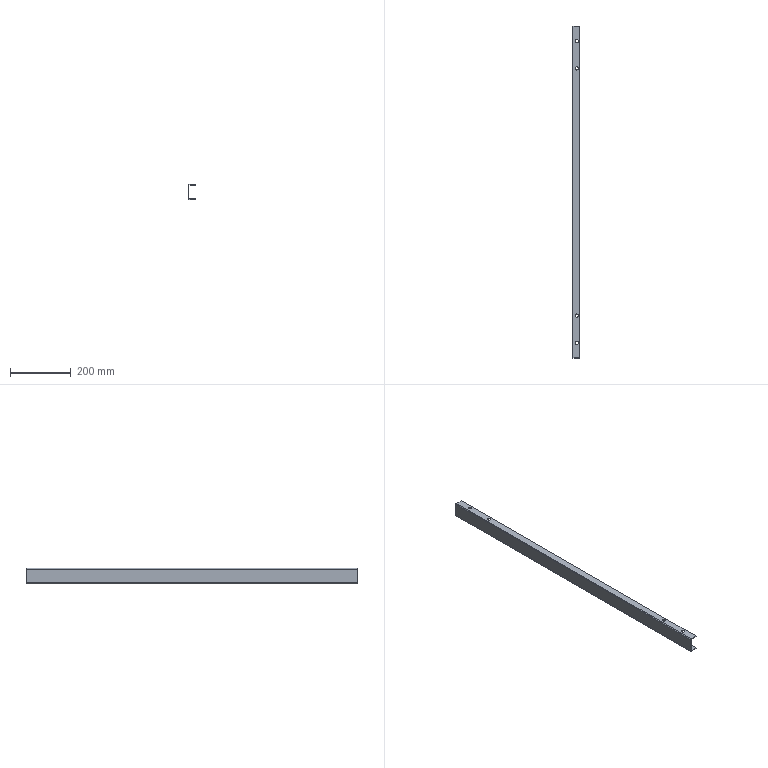Part | 1 solid | 38 faces | box 25 x 1096 x 50 mm | volume 206654 mm3 | cylinder 20 | plane 18 | commonest cylinder face diameters 11 x16 0.4 x2 4.4 x2
STEP:
#1=CARTESIAN_POINT('',(20.5,498.,-23.));
#2=VERTEX_POINT('',#1);
#3=CARTESIAN_POINT('',(9.5,498.,-23.));
#4=VERTEX_POINT('',#3);
#5=CARTESIAN_POINT('',(15.,498.,-23.));
#6=DIRECTION('',(0.,0.,-1.));
#7=DIRECTION('',(-1.,0.,0.));
#8=AXIS2_PLACEMENT_3D('',#5,#6,#7);
#9=CIRCLE('',#8,5.5);
#10=EDGE_CURVE('',#2,#4,#9,.T.);
#11=ORIENTED_EDGE('',*,*,#10,.F.);
#12=CARTESIAN_POINT('',(20.5,498.,-25.));
#13=VERTEX_POINT('',#12);
#14=CARTESIAN_POINT('',(20.5,498.,25.));
#15=DIRECTION('',(0.,0.,-1.));
#16=VECTOR('',#15,1000.);
#17=LINE('',#14,#16);
#18=EDGE_CURVE('',#2,#13,#17,.T.);
#19=ORIENTED_EDGE('',*,*,#18,.T.);
#20=CARTESIAN_POINT('',(9.5,498.,-25.));
#21=VERTEX_POINT('',#20);
#22=CARTESIAN_POINT('',(15.,498.,-25.));
#23=DIRECTION('',(0.,0.,-1.));
#24=DIRECTION('',(-1.,0.,0.));
#25=AXIS2_PLACEMENT_3D('',#22,#23,#24);
#26=CIRCLE('',#25,5.5);
#27=EDGE_CURVE('',#13,#21,#26,.T.);
#28=ORIENTED_EDGE('',*,*,#27,.T.);
#29=CARTESIAN_POINT('',(9.5,498.,25.));
#30=DIRECTION('',(0.,0.,-1.));
#31=VECTOR('',#30,1000.);
#32=LINE('',#29,#31);
#33=EDGE_CURVE('',#4,#21,#32,.T.);
#34=ORIENTED_EDGE('',*,*,#33,.F.);
#35=EDGE_LOOP('',(#11,#19,#28,#34));
#36=FACE_OUTER_BOUND('',#35,.T.);
#37=CARTESIAN_POINT('',(15.,498.,25.));
#38=DIRECTION('',(0.,0.,-1.));
#39=DIRECTION('',(-1.,0.,0.));
#40=AXIS2_PLACEMENT_3D('',#37,#38,#39);
#41=CYLINDRICAL_SURFACE('',#40,5.5);
#42=ADVANCED_FACE('',(#36),#41,.F.);
#43=CARTESIAN_POINT('',(20.5,408.,-23.));
#44=VERTEX_POINT('',#43);
#45=CARTESIAN_POINT('',(9.5,408.,-23.));
#46=VERTEX_POINT('',#45);
#47=CARTESIAN_POINT('',(15.,408.,-23.));
#48=DIRECTION('',(0.,0.,-1.));
#49=DIRECTION('',(-1.,0.,0.));
#50=AXIS2_PLACEMENT_3D('',#47,#48,#49);
#51=CIRCLE('',#50,5.5);
#52=EDGE_CURVE('',#44,#46,#51,.T.);
#53=ORIENTED_EDGE('',*,*,#52,.F.);
#54=CARTESIAN_POINT('',(20.5,408.,-25.));
#55=VERTEX_POINT('',#54);
#56=CARTESIAN_POINT('',(20.5,408.,25.));
#57=DIRECTION('',(0.,0.,-1.));
#58=VECTOR('',#57,1000.);
#59=LINE('',#56,#58);
#60=EDGE_CURVE('',#44,#55,#59,.T.);
#61=ORIENTED_EDGE('',*,*,#60,.T.);
#62=CARTESIAN_POINT('',(9.5,408.,-25.));
#63=VERTEX_POINT('',#62);
#64=CARTESIAN_POINT('',(15.,408.,-25.));
#65=DIRECTION('',(0.,0.,-1.));
#66=DIRECTION('',(-1.,0.,0.));
#67=AXIS2_PLACEMENT_3D('',#64,#65,#66);
#68=CIRCLE('',#67,5.5);
#69=EDGE_CURVE('',#55,#63,#68,.T.);
#70=ORIENTED_EDGE('',*,*,#69,.T.);
#71=CARTESIAN_POINT('',(9.5,408.,25.));
#72=DIRECTION('',(0.,0.,-1.));
#73=VECTOR('',#72,1000.);
#74=LINE('',#71,#73);
#75=EDGE_CURVE('',#46,#63,#74,.T.);
#76=ORIENTED_EDGE('',*,*,#75,.F.);
#77=EDGE_LOOP('',(#53,#61,#70,#76));
#78=FACE_OUTER_BOUND('',#77,.T.);
#79=CARTESIAN_POINT('',(15.,408.,25.));
#80=DIRECTION('',(0.,0.,-1.));
#81=DIRECTION('',(-1.,0.,0.));
#82=AXIS2_PLACEMENT_3D('',#79,#80,#81);
#83=CYLINDRICAL_SURFACE('',#82,5.5);
#84=ADVANCED_FACE('',(#78),#83,.F.);
#85=CARTESIAN_POINT('',(20.5,-408.,-23.));
#86=VERTEX_POINT('',#85);
#87=CARTESIAN_POINT('',(9.5,-408.,-23.));
#88=VERTEX_POINT('',#87);
#89=CARTESIAN_POINT('',(15.,-408.,-23.));
#90=DIRECTION('',(0.,0.,-1.));
#91=DIRECTION('',(-1.,0.,0.));
#92=AXIS2_PLACEMENT_3D('',#89,#90,#91);
#93=CIRCLE('',#92,5.5);
#94=EDGE_CURVE('',#86,#88,#93,.T.);
#95=ORIENTED_EDGE('',*,*,#94,.F.);
#96=CARTESIAN_POINT('',(20.5,-408.,-25.));
#97=VERTEX_POINT('',#96);
#98=CARTESIAN_POINT('',(20.5,-408.,25.));
#99=DIRECTION('',(0.,0.,-1.));
#100=VECTOR('',#99,1000.);
#101=LINE('',#98,#100);
#102=EDGE_CURVE('',#86,#97,#101,.T.);
#103=ORIENTED_EDGE('',*,*,#102,.T.);
#104=CARTESIAN_POINT('',(9.5,-408.,-25.));
#105=VERTEX_POINT('',#104);
#106=CARTESIAN_POINT('',(15.,-408.,-25.));
#107=DIRECTION('',(0.,0.,-1.));
#108=DIRECTION('',(-1.,0.,0.));
#109=AXIS2_PLACEMENT_3D('',#106,#107,#108);
#110=CIRCLE('',#109,5.5);
#111=EDGE_CURVE('',#97,#105,#110,.T.);
#112=ORIENTED_EDGE('',*,*,#111,.T.);
#113=CARTESIAN_POINT('',(9.5,-408.,25.));
#114=DIRECTION('',(0.,0.,-1.));
#115=VECTOR('',#114,1000.);
#116=LINE('',#113,#115);
#117=EDGE_CURVE('',#88,#105,#116,.T.);
#118=ORIENTED_EDGE('',*,*,#117,.F.);
#119=EDGE_LOOP('',(#95,#103,#112,#118));
#120=FACE_OUTER_BOUND('',#119,.T.);
#121=CARTESIAN_POINT('',(15.,-408.,25.));
#122=DIRECTION('',(0.,0.,-1.));
#123=DIRECTION('',(-1.,0.,0.));
#124=AXIS2_PLACEMENT_3D('',#121,#122,#123);
#125=CYLINDRICAL_SURFACE('',#124,5.5);
#126=ADVANCED_FACE('',(#120),#125,.F.);
#127=CARTESIAN_POINT('',(20.5,-498.,-23.));
#128=VERTEX_POINT('',#127);
#129=CARTESIAN_POINT('',(9.5,-498.,-23.));
#130=VERTEX_POINT('',#129);
#131=CARTESIAN_POINT('',(15.,-498.,-23.));
#132=DIRECTION('',(0.,0.,-1.));
#133=DIRECTION('',(-1.,0.,0.));
#134=AXIS2_PLACEMENT_3D('',#131,#132,#133);
#135=CIRCLE('',#134,5.5);
#136=EDGE_CURVE('',#128,#130,#135,.T.);
#137=ORIENTED_EDGE('',*,*,#136,.F.);
#138=CARTESIAN_POINT('',(20.5,-498.,-25.));
#139=VERTEX_POINT('',#138);
#140=CARTESIAN_POINT('',(20.5,-498.,25.));
#141=DIRECTION('',(0.,0.,-1.));
#142=VECTOR('',#141,1000.);
#143=LINE('',#140,#142);
#144=EDGE_CURVE('',#128,#139,#143,.T.);
#145=ORIENTED_EDGE('',*,*,#144,.T.);
#146=CARTESIAN_POINT('',(9.5,-498.,-25.));
#147=VERTEX_POINT('',#146);
#148=CARTESIAN_POINT('',(15.,-498.,-25.));
#149=DIRECTION('',(0.,0.,-1.));
#150=DIRECTION('',(-1.,0.,0.));
#151=AXIS2_PLACEMENT_3D('',#148,#149,#150);
#152=CIRCLE('',#151,5.5);
#153=EDGE_CURVE('',#139,#147,#152,.T.);
#154=ORIENTED_EDGE('',*,*,#153,.T.);
#155=CARTESIAN_POINT('',(9.5,-498.,25.));
#156=DIRECTION('',(0.,0.,-1.));
#157=VECTOR('',#156,1000.);
#158=LINE('',#155,#157);
#159=EDGE_CURVE('',#130,#147,#158,.T.);
#160=ORIENTED_EDGE('',*,*,#159,.F.);
#161=EDGE_LOOP('',(#137,#145,#154,#160));
#162=FACE_OUTER_BOUND('',#161,.T.);
#163=CARTESIAN_POINT('',(15.,-498.,25.));
#164=DIRECTION('',(0.,0.,-1.));
#165=DIRECTION('',(-1.,0.,0.));
#166=AXIS2_PLACEMENT_3D('',#163,#164,#165);
#167=CYLINDRICAL_SURFACE('',#166,5.5);
#168=ADVANCED_FACE('',(#162),#167,.F.);
#169=CARTESIAN_POINT('',(20.5,498.,25.));
#170=VERTEX_POINT('',#169);
#171=CARTESIAN_POINT('',(9.5,498.,25.));
#172=VERTEX_POINT('',#171);
#173=CARTESIAN_POINT('',(15.,498.,25.));
#174=DIRECTION('',(0.,0.,-1.));
#175=DIRECTION('',(-1.,0.,0.));
#176=AXIS2_PLACEMENT_3D('',#173,#174,#175);
#177=CIRCLE('',#176,5.5);
#178=EDGE_CURVE('',#170,#172,#177,.T.);
#179=ORIENTED_EDGE('',*,*,#178,.F.);
#180=CARTESIAN_POINT('',(20.5,498.,23.));
#181=VERTEX_POINT('',#180);
#182=CARTESIAN_POINT('',(20.5,498.,25.));
#183=DIRECTION('',(0.,0.,-1.));
#184=VECTOR('',#183,1000.);
#185=LINE('',#182,#184);
#186=EDGE_CURVE('',#170,#181,#185,.T.);
#187=ORIENTED_EDGE('',*,*,#186,.T.);
#188=CARTESIAN_POINT('',(9.5,498.,23.));
#189=VERTEX_POINT('',#188);
#190=CARTESIAN_POINT('',(15.,498.,23.));
#191=DIRECTION('',(0.,0.,1.));
#192=DIRECTION('',(1.,0.,0.));
#193=AXIS2_PLACEMENT_3D('',#190,#191,#192);
#194=CIRCLE('',#193,5.5);
#195=EDGE_CURVE('',#189,#181,#194,.T.);
#196=ORIENTED_EDGE('',*,*,#195,.F.);
#197=CARTESIAN_POINT('',(9.5,498.,25.));
#198=DIRECTION('',(0.,0.,-1.));
#199=VECTOR('',#198,1000.);
#200=LINE('',#197,#199);
#201=EDGE_CURVE('',#172,#189,#200,.T.);
#202=ORIENTED_EDGE('',*,*,#201,.F.);
#203=EDGE_LOOP('',(#179,#187,#196,#202));
#204=FACE_OUTER_BOUND('',#203,.T.);
#205=CARTESIAN_POINT('',(15.,498.,25.));
#206=DIRECTION('',(0.,0.,-1.));
#207=DIRECTION('',(-1.,0.,0.));
#208=AXIS2_PLACEMENT_3D('',#205,#206,#207);
#209=CYLINDRICAL_SURFACE('',#208,5.5);
#210=ADVANCED_FACE('',(#204),#209,.F.);
#211=CARTESIAN_POINT('',(20.5,408.,25.));
#212=VERTEX_POINT('',#211);
#213=CARTESIAN_POINT('',(9.5,408.,25.));
#214=VERTEX_POINT('',#213);
#215=CARTESIAN_POINT('',(15.,408.,25.));
#216=DIRECTION('',(0.,0.,-1.));
#217=DIRECTION('',(-1.,0.,0.));
#218=AXIS2_PLACEMENT_3D('',#215,#216,#217);
#219=CIRCLE('',#218,5.5);
#220=EDGE_CURVE('',#212,#214,#219,.T.);
#221=ORIENTED_EDGE('',*,*,#220,.F.);
#222=CARTESIAN_POINT('',(20.5,408.,23.));
#223=VERTEX_POINT('',#222);
#224=CARTESIAN_POINT('',(20.5,408.,25.));
#225=DIRECTION('',(0.,0.,-1.));
#226=VECTOR('',#225,1000.);
#227=LINE('',#224,#226);
#228=EDGE_CURVE('',#212,#223,#227,.T.);
#229=ORIENTED_EDGE('',*,*,#228,.T.);
#230=CARTESIAN_POINT('',(9.5,408.,23.));
#231=VERTEX_POINT('',#230);
#232=CARTESIAN_POINT('',(15.,408.,23.));
#233=DIRECTION('',(0.,0.,1.));
#234=DIRECTION('',(1.,0.,0.));
#235=AXIS2_PLACEMENT_3D('',#232,#233,#234);
#236=CIRCLE('',#235,5.5);
#237=EDGE_CURVE('',#231,#223,#236,.T.);
#238=ORIENTED_EDGE('',*,*,#237,.F.);
#239=CARTESIAN_POINT('',(9.5,408.,25.));
#240=DIRECTION('',(0.,0.,-1.));
#241=VECTOR('',#240,1000.);
#242=LINE('',#239,#241);
#243=EDGE_CURVE('',#214,#231,#242,.T.);
#244=ORIENTED_EDGE('',*,*,#243,.F.);
#245=EDGE_LOOP('',(#221,#229,#238,#244));
#246=FACE_OUTER_BOUND('',#245,.T.);
#247=CARTESIAN_POINT('',(15.,408.,25.));
#248=DIRECTION('',(0.,0.,-1.));
#249=DIRECTION('',(-1.,0.,0.));
#250=AXIS2_PLACEMENT_3D('',#247,#248,#249);
#251=CYLINDRICAL_SURFACE('',#250,5.5);
#252=ADVANCED_FACE('',(#246),#251,.F.);
#253=CARTESIAN_POINT('',(20.5,-408.,25.));
#254=VERTEX_POINT('',#253);
#255=CARTESIAN_POINT('',(9.5,-408.,25.));
#256=VERTEX_POINT('',#255);
#257=CARTESIAN_POINT('',(15.,-408.,25.));
#258=DIRECTION('',(0.,0.,-1.));
#259=DIRECTION('',(1.,0.,0.));
#260=AXIS2_PLACEMENT_3D('',#257,#258,#259);
#261=CIRCLE('',#260,5.5);
#262=EDGE_CURVE('',#254,#256,#261,.T.);
#263=ORIENTED_EDGE('',*,*,#262,.F.);
#264=CARTESIAN_POINT('',(20.5,-408.,23.));
#265=VERTEX_POINT('',#264);
#266=CARTESIAN_POINT('',(20.5,-408.,25.));
#267=DIRECTION('',(0.,0.,-1.));
#268=VECTOR('',#267,1000.);
#269=LINE('',#266,#268);
#270=EDGE_CURVE('',#254,#265,#269,.T.);
#271=ORIENTED_EDGE('',*,*,#270,.T.);
#272=CARTESIAN_POINT('',(9.5,-408.,23.));
#273=VERTEX_POINT('',#272);
#274=CARTESIAN_POINT('',(15.,-408.,23.));
#275=DIRECTION('',(0.,0.,1.));
#276=DIRECTION('',(1.,0.,0.));
#277=AXIS2_PLACEMENT_3D('',#274,#275,#276);
#278=CIRCLE('',#277,5.5);
#279=EDGE_CURVE('',#273,#265,#278,.T.);
#280=ORIENTED_EDGE('',*,*,#279,.F.);
#281=CARTESIAN_POINT('',(9.5,-408.,25.));
#282=DIRECTION('',(0.,0.,-1.));
#283=VECTOR('',#282,1000.);
#284=LINE('',#281,#283);
#285=EDGE_CURVE('',#256,#273,#284,.T.);
#286=ORIENTED_EDGE('',*,*,#285,.F.);
#287=EDGE_LOOP('',(#263,#271,#280,#286));
#288=FACE_OUTER_BOUND('',#287,.T.);
#289=CARTESIAN_POINT('',(15.,-408.,25.));
#290=DIRECTION('',(0.,0.,-1.));
#291=DIRECTION('',(-1.,0.,0.));
#292=AXIS2_PLACEMENT_3D('',#289,#290,#291);
#293=CYLINDRICAL_SURFACE('',#292,5.5);
#294=ADVANCED_FACE('',(#288),#293,.F.);
#295=CARTESIAN_POINT('',(20.5,-498.,25.));
#296=VERTEX_POINT('',#295);
#297=CARTESIAN_POINT('',(9.5,-498.,25.));
#298=VERTEX_POINT('',#297);
#299=CARTESIAN_POINT('',(15.,-498.,25.));
#300=DIRECTION('',(0.,0.,-1.));
#301=DIRECTION('',(1.,0.,0.));
#302=AXIS2_PLACEMENT_3D('',#299,#300,#301);
#303=CIRCLE('',#302,5.5);
#304=EDGE_CURVE('',#296,#298,#303,.T.);
#305=ORIENTED_EDGE('',*,*,#304,.F.);
#306=CARTESIAN_POINT('',(20.5,-498.,23.));
#307=VERTEX_POINT('',#306);
#308=CARTESIAN_POINT('',(20.5,-498.,25.));
#309=DIRECTION('',(0.,0.,-1.));
#310=VECTOR('',#309,1000.);
#311=LINE('',#308,#310);
#312=EDGE_CURVE('',#296,#307,#311,.T.);
#313=ORIENTED_EDGE('',*,*,#312,.T.);
#314=CARTESIAN_POINT('',(9.5,-498.,23.));
#315=VERTEX_POINT('',#314);
#316=CARTESIAN_POINT('',(15.,-498.,23.));
#317=DIRECTION('',(0.,0.,1.));
#318=DIRECTION('',(1.,0.,0.));
#319=AXIS2_PLACEMENT_3D('',#316,#317,#318);
#320=CIRCLE('',#319,5.5);
#321=EDGE_CURVE('',#315,#307,#320,.T.);
#322=ORIENTED_EDGE('',*,*,#321,.F.);
#323=CARTESIAN_POINT('',(9.5,-498.,25.));
#324=DIRECTION('',(0.,0.,-1.));
#325=VECTOR('',#324,1000.);
#326=LINE('',#323,#325);
#327=EDGE_CURVE('',#298,#315,#326,.T.);
#328=ORIENTED_EDGE('',*,*,#327,.F.);
#329=EDGE_LOOP('',(#305,#313,#322,#328));
#330=FACE_OUTER_BOUND('',#329,.T.);
#331=CARTESIAN_POINT('',(15.,-498.,25.));
#332=DIRECTION('',(0.,0.,-1.));
#333=DIRECTION('',(-1.,0.,0.));
#334=AXIS2_PLACEMENT_3D('',#331,#332,#333);
#335=CYLINDRICAL_SURFACE('',#334,5.5);
#336=ADVANCED_FACE('',(#330),#335,.F.);
#337=CARTESIAN_POINT('',(0.,548.,22.8));
#338=VERTEX_POINT('',#337);
#339=CARTESIAN_POINT('',(2.,548.,22.8));
#340=VERTEX_POINT('',#339);
#341=CARTESIAN_POINT('',(0.,548.,22.8));
#342=DIRECTION('',(1.,0.,0.));
#343=VECTOR('',#342,1000.);
#344=LINE('',#341,#343);
#345=EDGE_CURVE('',#338,#340,#344,.T.);
#346=ORIENTED_EDGE('',*,*,#345,.F.);
#347=CARTESIAN_POINT('',(2.2,548.,25.));
#348=VERTEX_POINT('',#347);
#349=CARTESIAN_POINT('',(2.2,548.,22.8));
#350=DIRECTION('',(0.,-1.,0.));
#351=DIRECTION('',(0.,0.,1.));
#352=AXIS2_PLACEMENT_3D('',#349,#350,#351);
#353=CIRCLE('',#352,2.2);
#354=EDGE_CURVE('',#348,#338,#353,.T.);
#355=ORIENTED_EDGE('',*,*,#354,.F.);
#356=CARTESIAN_POINT('',(2.2,548.,23.));
#357=VERTEX_POINT('',#356);
#358=CARTESIAN_POINT('',(2.2,548.,23.));
#359=DIRECTION('',(0.,0.,1.));
#360=VECTOR('',#359,1000.);
#361=LINE('',#358,#360);
#362=EDGE_CURVE('',#357,#348,#361,.T.);
#363=ORIENTED_EDGE('',*,*,#362,.F.);
#364=CARTESIAN_POINT('',(2.2,548.,22.8));
#365=DIRECTION('',(0.,-1.,0.));
#366=DIRECTION('',(1.,0.,0.));
#367=AXIS2_PLACEMENT_3D('',#364,#365,#366);
#368=CIRCLE('',#367,0.2);
#369=EDGE_CURVE('',#357,#340,#368,.T.);
#370=ORIENTED_EDGE('',*,*,#369,.T.);
#371=EDGE_LOOP('',(#346,#355,#363,#370));
#372=FACE_OUTER_BOUND('',#371,.T.);
#373=CARTESIAN_POINT('',(0.,548.,22.8));
#374=DIRECTION('',(0.,1.,0.));
#375=DIRECTION('',(0.,0.,1.));
#376=AXIS2_PLACEMENT_3D('',#373,#374,#375);
#377=PLANE('',#376);
#378=ADVANCED_FACE('',(#372),#377,.T.);
#379=CARTESIAN_POINT('',(0.,548.,-22.8));
#380=VERTEX_POINT('',#379);
#381=CARTESIAN_POINT('',(0.,548.,-25.));
#382=DIRECTION('',(0.,0.,-1.));
#383=VECTOR('',#382,1000.);
#384=LINE('',#381,#383);
#385=EDGE_CURVE('',#338,#380,#384,.T.);
#386=ORIENTED_EDGE('',*,*,#385,.F.);
#387=ORIENTED_EDGE('',*,*,#345,.T.);
#388=CARTESIAN_POINT('',(2.,548.,-22.8));
#389=VERTEX_POINT('',#388);
#390=CARTESIAN_POINT('',(2.,548.,-25.));
#391=DIRECTION('',(0.,0.,-1.));
#392=VECTOR('',#391,1000.);
#393=LINE('',#390,#392);
#394=EDGE_CURVE('',#340,#389,#393,.T.);
#395=ORIENTED_EDGE('',*,*,#394,.T.);
#396=CARTESIAN_POINT('',(2.,548.,-22.8));
#397=DIRECTION('',(-1.,0.,0.));
#398=VECTOR('',#397,1000.);
#399=LINE('',#396,#398);
#400=EDGE_CURVE('',#389,#380,#399,.T.);
#401=ORIENTED_EDGE('',*,*,#400,.T.);
#402=EDGE_LOOP('',(#386,#387,#395,#401));
#403=FACE_OUTER_BOUND('',#402,.T.);
#404=CARTESIAN_POINT('',(2.2,548.,23.));
#405=DIRECTION('',(0.,1.,0.));
#406=DIRECTION('',(0.,0.,1.));
#407=AXIS2_PLACEMENT_3D('',#404,#405,#406);
#408=PLANE('',#407);
#409=ADVANCED_FACE('',(#403),#408,.T.);
#410=CARTESIAN_POINT('',(2.2,-548.,25.));
#411=VERTEX_POINT('',#410);
#412=CARTESIAN_POINT('',(2.2,-548.,23.));
#413=VERTEX_POINT('',#412);
#414=CARTESIAN_POINT('',(2.2,-548.,25.));
#415=DIRECTION('',(0.,0.,-1.));
#416=VECTOR('',#415,1000.);
#417=LINE('',#414,#416);
#418=EDGE_CURVE('',#411,#413,#417,.T.);
#419=ORIENTED_EDGE('',*,*,#418,.F.);
#420=CARTESIAN_POINT('',(0.,-548.,22.8));
#421=VERTEX_POINT('',#420);
#422=CARTESIAN_POINT('',(2.2,-548.,22.8));
#423=DIRECTION('',(0.,-1.,0.));
#424=DIRECTION('',(0.,0.,1.));
#425=AXIS2_PLACEMENT_3D('',#422,#423,#424);
#426=CIRCLE('',#425,2.2);
#427=EDGE_CURVE('',#411,#421,#426,.T.);
#428=ORIENTED_EDGE('',*,*,#427,.T.);
#429=CARTESIAN_POINT('',(2.,-548.,22.8));
#430=VERTEX_POINT('',#429);
#431=CARTESIAN_POINT('',(2.,-548.,22.8));
#432=DIRECTION('',(-1.,0.,0.));
#433=VECTOR('',#432,1000.);
#434=LINE('',#431,#433);
#435=EDGE_CURVE('',#430,#421,#434,.T.);
#436=ORIENTED_EDGE('',*,*,#435,.F.);
#437=CARTESIAN_POINT('',(2.2,-548.,22.8));
#438=DIRECTION('',(0.,-1.,0.));
#439=DIRECTION('',(1.,0.,0.));
#440=AXIS2_PLACEMENT_3D('',#437,#438,#439);
#441=CIRCLE('',#440,0.2);
#442=EDGE_CURVE('',#413,#430,#441,.T.);
#443=ORIENTED_EDGE('',*,*,#442,.F.);
#444=EDGE_LOOP('',(#419,#428,#436,#443));
#445=FACE_OUTER_BOUND('',#444,.T.);
#446=CARTESIAN_POINT('',(2.2,-548.,25.));
#447=DIRECTION('',(0.,-1.,0.));
#448=DIRECTION('',(0.,0.,-1.));
#449=AXIS2_PLACEMENT_3D('',#446,#447,#448);
#450=PLANE('',#449);
#451=ADVANCED_FACE('',(#445),#450,.T.);
#452=CARTESIAN_POINT('',(25.,-548.,25.));
#453=VERTEX_POINT('',#452);
#454=CARTESIAN_POINT('',(0.,-548.,25.));
#455=DIRECTION('',(-1.,0.,0.));
#456=VECTOR('',#455,1000.);
#457=LINE('',#454,#456);
#458=EDGE_CURVE('',#453,#411,#457,.T.);
#459=ORIENTED_EDGE('',*,*,#458,.T.);
#460=ORIENTED_EDGE('',*,*,#418,.T.);
#461=CARTESIAN_POINT('',(25.,-548.,23.));
#462=VERTEX_POINT('',#461);
#463=CARTESIAN_POINT('',(0.,-548.,23.));
#464=DIRECTION('',(-1.,0.,0.));
#465=VECTOR('',#464,1000.);
#466=LINE('',#463,#465);
#467=EDGE_CURVE('',#462,#413,#466,.T.);
#468=ORIENTED_EDGE('',*,*,#467,.F.);
#469=CARTESIAN_POINT('',(25.,-548.,23.));
#470=DIRECTION('',(0.,0.,1.));
#471=VECTOR('',#470,1000.);
#472=LINE('',#469,#471);
#473=EDGE_CURVE('',#462,#453,#472,.T.);
#474=ORIENTED_EDGE('',*,*,#473,.T.);
#475=EDGE_LOOP('',(#459,#460,#468,#474));
#476=FACE_OUTER_BOUND('',#475,.T.);
#477=CARTESIAN_POINT('',(2.,-548.,22.8));
#478=DIRECTION('',(0.,-1.,0.));
#479=DIRECTION('',(0.,0.,-1.));
#480=AXIS2_PLACEMENT_3D('',#477,#478,#479);
#481=PLANE('',#480);
#482=ADVANCED_FACE('',(#476),#481,.T.);
#483=CARTESIAN_POINT('',(2.2,548.,-25.));
#484=VERTEX_POINT('',#483);
#485=CARTESIAN_POINT('',(2.2,548.,-23.));
#486=VERTEX_POINT('',#485);
#487=CARTESIAN_POINT('',(2.2,548.,-25.));
#488=DIRECTION('',(0.,0.,1.));
#489=VECTOR('',#488,1000.);
#490=LINE('',#487,#489);
#491=EDGE_CURVE('',#484,#486,#490,.T.);
#492=ORIENTED_EDGE('',*,*,#491,.F.);
#493=CARTESIAN_POINT('',(2.2,548.,-22.8));
#494=DIRECTION('',(0.,-1.,0.));
#495=DIRECTION('',(0.,0.,1.));
#496=AXIS2_PLACEMENT_3D('',#493,#494,#495);
#497=CIRCLE('',#496,2.2);
#498=EDGE_CURVE('',#380,#484,#497,.T.);
#499=ORIENTED_EDGE('',*,*,#498,.F.);
#500=ORIENTED_EDGE('',*,*,#400,.F.);
#501=CARTESIAN_POINT('',(2.2,548.,-22.8));
#502=DIRECTION('',(0.,-1.,0.));
#503=DIRECTION('',(1.,0.,0.));
#504=AXIS2_PLACEMENT_3D('',#501,#502,#503);
#505=CIRCLE('',#504,0.2);
#506=EDGE_CURVE('',#389,#486,#505,.T.);
#507=ORIENTED_EDGE('',*,*,#506,.T.);
#508=EDGE_LOOP('',(#492,#499,#500,#507));
#509=FACE_OUTER_BOUND('',#508,.T.);
#510=CARTESIAN_POINT('',(2.2,548.,-25.));
#511=DIRECTION('',(0.,1.,0.));
#512=DIRECTION('',(0.,0.,1.));
#513=AXIS2_PLACEMENT_3D('',#510,#511,#512);
#514=PLANE('',#513);
#515=ADVANCED_FACE('',(#509),#514,.T.);
#516=CARTESIAN_POINT('',(25.,548.,-25.));
#517=VERTEX_POINT('',#516);
#518=CARTESIAN_POINT('',(0.,548.,-25.));
#519=DIRECTION('',(1.,0.,0.));
#520=VECTOR('',#519,1000.);
#521=LINE('',#518,#520);
#522=EDGE_CURVE('',#484,#517,#521,.T.);
#523=ORIENTED_EDGE('',*,*,#522,.F.);
#524=ORIENTED_EDGE('',*,*,#491,.T.);
#525=CARTESIAN_POINT('',(25.,548.,-23.));
#526=VERTEX_POINT('',#525);
#527=CARTESIAN_POINT('',(0.,548.,-23.));
#528=DIRECTION('',(1.,0.,0.));
#529=VECTOR('',#528,1000.);
#530=LINE('',#527,#529);
#531=EDGE_CURVE('',#486,#526,#530,.T.);
#532=ORIENTED_EDGE('',*,*,#531,.T.);
#533=CARTESIAN_POINT('',(25.,548.,-25.));
#534=DIRECTION('',(0.,0.,1.));
#535=VECTOR('',#534,1000.);
#536=LINE('',#533,#535);
#537=EDGE_CURVE('',#517,#526,#536,.T.);
#538=ORIENTED_EDGE('',*,*,#537,.F.);
#539=EDGE_LOOP('',(#523,#524,#532,#538));
#540=FACE_OUTER_BOUND('',#539,.T.);
#541=CARTESIAN_POINT('',(2.,548.,-22.8));
#542=DIRECTION('',(0.,1.,0.));
#543=DIRECTION('',(0.,0.,1.));
#544=AXIS2_PLACEMENT_3D('',#541,#542,#543);
#545=PLANE('',#544);
#546=ADVANCED_FACE('',(#540),#545,.T.);
#547=CARTESIAN_POINT('',(0.,-548.,-22.8));
#548=VERTEX_POINT('',#547);
#549=CARTESIAN_POINT('',(2.,-548.,-22.8));
#550=VERTEX_POINT('',#549);
#551=CARTESIAN_POINT('',(0.,-548.,-22.8));
#552=DIRECTION('',(1.,0.,0.));
#553=VECTOR('',#552,1000.);
#554=LINE('',#551,#553);
#555=EDGE_CURVE('',#548,#550,#554,.T.);
#556=ORIENTED_EDGE('',*,*,#555,.F.);
#557=CARTESIAN_POINT('',(2.2,-548.,-25.));
#558=VERTEX_POINT('',#557);
#559=CARTESIAN_POINT('',(2.2,-548.,-22.8));
#560=DIRECTION('',(0.,-1.,0.));
#561=DIRECTION('',(0.,0.,1.));
#562=AXIS2_PLACEMENT_3D('',#559,#560,#561);
#563=CIRCLE('',#562,2.2);
#564=EDGE_CURVE('',#548,#558,#563,.T.);
#565=ORIENTED_EDGE('',*,*,#564,.T.);
#566=CARTESIAN_POINT('',(2.2,-548.,-23.));
#567=VERTEX_POINT('',#566);
#568=CARTESIAN_POINT('',(2.2,-548.,-23.));
#569=DIRECTION('',(0.,0.,-1.));
#570=VECTOR('',#569,1000.);
#571=LINE('',#568,#570);
#572=EDGE_CURVE('',#567,#558,#571,.T.);
#573=ORIENTED_EDGE('',*,*,#572,.F.);
#574=CARTESIAN_POINT('',(2.2,-548.,-22.8));
#575=DIRECTION('',(0.,-1.,0.));
#576=DIRECTION('',(1.,0.,0.));
#577=AXIS2_PLACEMENT_3D('',#574,#575,#576);
#578=CIRCLE('',#577,0.2);
#579=EDGE_CURVE('',#550,#567,#578,.T.);
#580=ORIENTED_EDGE('',*,*,#579,.F.);
#581=EDGE_LOOP('',(#556,#565,#573,#580));
#582=FACE_OUTER_BOUND('',#581,.T.);
#583=CARTESIAN_POINT('',(0.,-548.,-22.8));
#584=DIRECTION('',(0.,-1.,0.));
#585=DIRECTION('',(0.,0.,-1.));
#586=AXIS2_PLACEMENT_3D('',#583,#584,#585);
#587=PLANE('',#586);
#588=ADVANCED_FACE('',(#582),#587,.T.);
#589=CARTESIAN_POINT('',(0.,-548.,-25.));
#590=DIRECTION('',(0.,0.,-1.));
#591=VECTOR('',#590,1000.);
#592=LINE('',#589,#591);
#593=EDGE_CURVE('',#421,#548,#592,.T.);
#594=ORIENTED_EDGE('',*,*,#593,.T.);
#595=ORIENTED_EDGE('',*,*,#555,.T.);
#596=CARTESIAN_POINT('',(2.,-548.,-25.));
#597=DIRECTION('',(0.,0.,-1.));
#598=VECTOR('',#597,1000.);
#599=LINE('',#596,#598);
#600=EDGE_CURVE('',#430,#550,#599,.T.);
#601=ORIENTED_EDGE('',*,*,#600,.F.);
#602=ORIENTED_EDGE('',*,*,#435,.T.);
#603=EDGE_LOOP('',(#594,#595,#601,#602));
#604=FACE_OUTER_BOUND('',#603,.T.);
#605=CARTESIAN_POINT('',(2.2,-548.,-23.));
#606=DIRECTION('',(0.,-1.,0.));
#607=DIRECTION('',(0.,0.,-1.));
#608=AXIS2_PLACEMENT_3D('',#605,#606,#607);
#609=PLANE('',#608);
#610=ADVANCED_FACE('',(#604),#609,.T.);
#611=CARTESIAN_POINT('',(15.,498.,-23.));
#612=DIRECTION('',(0.,0.,-1.));
#613=DIRECTION('',(-1.,0.,0.));
#614=AXIS2_PLACEMENT_3D('',#611,#612,#613);
#615=CIRCLE('',#614,5.5);
#616=EDGE_CURVE('',#4,#2,#615,.T.);
#617=ORIENTED_EDGE('',*,*,#616,.T.);
#618=ORIENTED_EDGE('',*,*,#10,.T.);
#619=EDGE_LOOP('',(#617,#618));
#620=FACE_BOUND('',#619,.T.);
#621=CARTESIAN_POINT('',(15.,408.,-23.));
#622=DIRECTION('',(0.,0.,-1.));
#623=DIRECTION('',(-1.,0.,0.));
#624=AXIS2_PLACEMENT_3D('',#621,#622,#623);
#625=CIRCLE('',#624,5.5);
#626=EDGE_CURVE('',#46,#44,#625,.T.);
#627=ORIENTED_EDGE('',*,*,#626,.T.);
#628=ORIENTED_EDGE('',*,*,#52,.T.);
#629=EDGE_LOOP('',(#627,#628));
#630=FACE_BOUND('',#629,.T.);
#631=CARTESIAN_POINT('',(15.,-408.,-23.));
#632=DIRECTION('',(0.,0.,-1.));
#633=DIRECTION('',(-1.,0.,0.));
#634=AXIS2_PLACEMENT_3D('',#631,#632,#633);
#635=CIRCLE('',#634,5.5);
#636=EDGE_CURVE('',#88,#86,#635,.T.);
#637=ORIENTED_EDGE('',*,*,#636,.T.);
#638=ORIENTED_EDGE('',*,*,#94,.T.);
#639=EDGE_LOOP('',(#637,#638));
#640=FACE_BOUND('',#639,.T.);
#641=CARTESIAN_POINT('',(15.,-498.,-23.));
#642=DIRECTION('',(0.,0.,-1.));
#643=DIRECTION('',(-1.,0.,0.));
#644=AXIS2_PLACEMENT_3D('',#641,#642,#643);
#645=CIRCLE('',#644,5.5);
#646=EDGE_CURVE('',#130,#128,#645,.T.);
#647=ORIENTED_EDGE('',*,*,#646,.T.);
#648=ORIENTED_EDGE('',*,*,#136,.T.);
#649=EDGE_LOOP('',(#647,#648));
#650=FACE_BOUND('',#649,.T.);
#651=CARTESIAN_POINT('',(25.,-548.,-23.));
#652=VERTEX_POINT('',#651);
#653=CARTESIAN_POINT('',(0.,-548.,-23.));
#654=DIRECTION('',(1.,0.,0.));
#655=VECTOR('',#654,1000.);
#656=LINE('',#653,#655);
#657=EDGE_CURVE('',#567,#652,#656,.T.);
#658=ORIENTED_EDGE('',*,*,#657,.T.);
#659=CARTESIAN_POINT('',(25.,548.,-23.));
#660=DIRECTION('',(0.,-1.,0.));
#661=VECTOR('',#660,1000.);
#662=LINE('',#659,#661);
#663=EDGE_CURVE('',#526,#652,#662,.T.);
#664=ORIENTED_EDGE('',*,*,#663,.F.);
#665=ORIENTED_EDGE('',*,*,#531,.F.);
#666=CARTESIAN_POINT('',(2.2,548.,-23.));
#667=DIRECTION('',(0.,-1.,0.));
#668=VECTOR('',#667,1000.);
#669=LINE('',#666,#668);
#670=EDGE_CURVE('',#486,#567,#669,.T.);
#671=ORIENTED_EDGE('',*,*,#670,.T.);
#672=EDGE_LOOP('',(#658,#664,#665,#671));
#673=FACE_OUTER_BOUND('',#672,.T.);
#674=CARTESIAN_POINT('',(0.,548.,-23.));
#675=DIRECTION('',(0.,0.,-1.));
#676=DIRECTION('',(-1.,0.,0.));
#677=AXIS2_PLACEMENT_3D('',#674,#675,#676);
#678=PLANE('',#677);
#679=ADVANCED_FACE('',(#620,#630,#640,#650,#673),#678,.F.);
#680=CARTESIAN_POINT('',(25.,-548.,-25.));
#681=VERTEX_POINT('',#680);
#682=CARTESIAN_POINT('',(25.,-548.,-25.));
#683=DIRECTION('',(0.,0.,1.));
#684=VECTOR('',#683,1000.);
#685=LINE('',#682,#684);
#686=EDGE_CURVE('',#681,#652,#685,.T.);
#687=ORIENTED_EDGE('',*,*,#686,.F.);
#688=CARTESIAN_POINT('',(25.,548.,-25.));
#689=DIRECTION('',(0.,-1.,0.));
#690=VECTOR('',#689,1000.);
#691=LINE('',#688,#690);
#692=EDGE_CURVE('',#517,#681,#691,.T.);
#693=ORIENTED_EDGE('',*,*,#692,.F.);
#694=ORIENTED_EDGE('',*,*,#537,.T.);
#695=ORIENTED_EDGE('',*,*,#663,.T.);
#696=EDGE_LOOP('',(#687,#693,#694,#695));
#697=FACE_OUTER_BOUND('',#696,.T.);
#698=CARTESIAN_POINT('',(25.,548.,-25.));
#699=DIRECTION('',(1.,0.,0.));
#700=DIRECTION('',(0.,0.,-1.));
#701=AXIS2_PLACEMENT_3D('',#698,#699,#700);
#702=PLANE('',#701);
#703=ADVANCED_FACE('',(#697),#702,.T.);
#704=CARTESIAN_POINT('',(15.,498.,-25.));
#705=DIRECTION('',(0.,0.,-1.));
#706=DIRECTION('',(-1.,0.,0.));
#707=AXIS2_PLACEMENT_3D('',#704,#705,#706);
#708=CIRCLE('',#707,5.5);
#709=EDGE_CURVE('',#21,#13,#708,.T.);
#710=ORIENTED_EDGE('',*,*,#709,.F.);
#711=ORIENTED_EDGE('',*,*,#27,.F.);
#712=EDGE_LOOP('',(#710,#711));
#713=FACE_BOUND('',#712,.T.);
#714=CARTESIAN_POINT('',(15.,408.,-25.));
#715=DIRECTION('',(0.,0.,-1.));
#716=DIRECTION('',(-1.,0.,0.));
#717=AXIS2_PLACEMENT_3D('',#714,#715,#716);
#718=CIRCLE('',#717,5.5);
#719=EDGE_CURVE('',#63,#55,#718,.T.);
#720=ORIENTED_EDGE('',*,*,#719,.F.);
#721=ORIENTED_EDGE('',*,*,#69,.F.);
#722=EDGE_LOOP('',(#720,#721));
#723=FACE_BOUND('',#722,.T.);
#724=CARTESIAN_POINT('',(15.,-408.,-25.));
#725=DIRECTION('',(0.,0.,-1.));
#726=DIRECTION('',(-1.,0.,0.));
#727=AXIS2_PLACEMENT_3D('',#724,#725,#726);
#728=CIRCLE('',#727,5.5);
#729=EDGE_CURVE('',#105,#97,#728,.T.);
#730=ORIENTED_EDGE('',*,*,#729,.F.);
#731=ORIENTED_EDGE('',*,*,#111,.F.);
#732=EDGE_LOOP('',(#730,#731));
#733=FACE_BOUND('',#732,.T.);
#734=CARTESIAN_POINT('',(15.,-498.,-25.));
#735=DIRECTION('',(0.,0.,-1.));
#736=DIRECTION('',(-1.,0.,0.));
#737=AXIS2_PLACEMENT_3D('',#734,#735,#736);
#738=CIRCLE('',#737,5.5);
#739=EDGE_CURVE('',#147,#139,#738,.T.);
#740=ORIENTED_EDGE('',*,*,#739,.F.);
#741=ORIENTED_EDGE('',*,*,#153,.F.);
#742=EDGE_LOOP('',(#740,#741));
#743=FACE_BOUND('',#742,.T.);
#744=CARTESIAN_POINT('',(0.,-548.,-25.));
#745=DIRECTION('',(1.,0.,0.));
#746=VECTOR('',#745,1000.);
#747=LINE('',#744,#746);
#748=EDGE_CURVE('',#558,#681,#747,.T.);
#749=ORIENTED_EDGE('',*,*,#748,.F.);
#750=CARTESIAN_POINT('',(2.2,548.,-25.));
#751=DIRECTION('',(0.,-1.,0.));
#752=VECTOR('',#751,1000.);
#753=LINE('',#750,#752);
#754=EDGE_CURVE('',#484,#558,#753,.T.);
#755=ORIENTED_EDGE('',*,*,#754,.F.);
#756=ORIENTED_EDGE('',*,*,#522,.T.);
#757=ORIENTED_EDGE('',*,*,#692,.T.);
#758=EDGE_LOOP('',(#749,#755,#756,#757));
#759=FACE_OUTER_BOUND('',#758,.T.);
#760=CARTESIAN_POINT('',(0.,548.,-25.));
#761=DIRECTION('',(0.,0.,-1.));
#762=DIRECTION('',(-1.,0.,0.));
#763=AXIS2_PLACEMENT_3D('',#760,#761,#762);
#764=PLANE('',#763);
#765=ADVANCED_FACE('',(#713,#723,#733,#743,#759),#764,.T.);
#766=ORIENTED_EDGE('',*,*,#564,.F.);
#767=CARTESIAN_POINT('',(0.,548.,-22.8));
#768=DIRECTION('',(0.,-1.,0.));
#769=VECTOR('',#768,1000.);
#770=LINE('',#767,#769);
#771=EDGE_CURVE('',#380,#548,#770,.T.);
#772=ORIENTED_EDGE('',*,*,#771,.F.);
#773=ORIENTED_EDGE('',*,*,#498,.T.);
#774=ORIENTED_EDGE('',*,*,#754,.T.);
#775=EDGE_LOOP('',(#766,#772,#773,#774));
#776=FACE_OUTER_BOUND('',#775,.T.);
#777=CARTESIAN_POINT('',(2.2,548.,-22.8));
#778=DIRECTION('',(0.,-1.,0.));
#779=DIRECTION('',(0.,0.,-1.));
#780=AXIS2_PLACEMENT_3D('',#777,#778,#779);
#781=CYLINDRICAL_SURFACE('',#780,2.2);
#782=ADVANCED_FACE('',(#776),#781,.T.);
#783=ORIENTED_EDGE('',*,*,#593,.F.);
#784=CARTESIAN_POINT('',(0.,548.,22.8));
#785=DIRECTION('',(0.,-1.,0.));
#786=VECTOR('',#785,1000.);
#787=LINE('',#784,#786);
#788=EDGE_CURVE('',#338,#421,#787,.T.);
#789=ORIENTED_EDGE('',*,*,#788,.F.);
#790=ORIENTED_EDGE('',*,*,#385,.T.);
#791=ORIENTED_EDGE('',*,*,#771,.T.);
#792=EDGE_LOOP('',(#783,#789,#790,#791));
#793=FACE_OUTER_BOUND('',#792,.T.);
#794=CARTESIAN_POINT('',(0.,548.,-25.));
#795=DIRECTION('',(-1.,0.,0.));
#796=DIRECTION('',(0.,0.,1.));
#797=AXIS2_PLACEMENT_3D('',#794,#795,#796);
#798=PLANE('',#797);
#799=ADVANCED_FACE('',(#793),#798,.T.);
#800=ORIENTED_EDGE('',*,*,#427,.F.);
#801=CARTESIAN_POINT('',(2.2,548.,25.));
#802=DIRECTION('',(0.,-1.,0.));
#803=VECTOR('',#802,1000.);
#804=LINE('',#801,#803);
#805=EDGE_CURVE('',#348,#411,#804,.T.);
#806=ORIENTED_EDGE('',*,*,#805,.F.);
#807=ORIENTED_EDGE('',*,*,#354,.T.);
#808=ORIENTED_EDGE('',*,*,#788,.T.);
#809=EDGE_LOOP('',(#800,#806,#807,#808));
#810=FACE_OUTER_BOUND('',#809,.T.);
#811=CARTESIAN_POINT('',(2.2,548.,22.8));
#812=DIRECTION('',(0.,-1.,0.));
#813=DIRECTION('',(0.,0.,-1.));
#814=AXIS2_PLACEMENT_3D('',#811,#812,#813);
#815=CYLINDRICAL_SURFACE('',#814,2.2);
#816=ADVANCED_FACE('',(#810),#815,.T.);
#817=CARTESIAN_POINT('',(15.,498.,25.));
#818=DIRECTION('',(0.,0.,-1.));
#819=DIRECTION('',(-1.,0.,0.));
#820=AXIS2_PLACEMENT_3D('',#817,#818,#819);
#821=CIRCLE('',#820,5.5);
#822=EDGE_CURVE('',#172,#170,#821,.T.);
#823=ORIENTED_EDGE('',*,*,#822,.T.);
#824=ORIENTED_EDGE('',*,*,#178,.T.);
#825=EDGE_LOOP('',(#823,#824));
#826=FACE_BOUND('',#825,.T.);
#827=CARTESIAN_POINT('',(15.,408.,25.));
#828=DIRECTION('',(0.,0.,-1.));
#829=DIRECTION('',(-1.,0.,0.));
#830=AXIS2_PLACEMENT_3D('',#827,#828,#829);
#831=CIRCLE('',#830,5.5);
#832=EDGE_CURVE('',#214,#212,#831,.T.);
#833=ORIENTED_EDGE('',*,*,#832,.T.);
#834=ORIENTED_EDGE('',*,*,#220,.T.);
#835=EDGE_LOOP('',(#833,#834));
#836=FACE_BOUND('',#835,.T.);
#837=CARTESIAN_POINT('',(15.,-408.,25.));
#838=DIRECTION('',(0.,0.,-1.));
#839=DIRECTION('',(1.,0.,0.));
#840=AXIS2_PLACEMENT_3D('',#837,#838,#839);
#841=CIRCLE('',#840,5.5);
#842=EDGE_CURVE('',#256,#254,#841,.T.);
#843=ORIENTED_EDGE('',*,*,#842,.T.);
#844=ORIENTED_EDGE('',*,*,#262,.T.);
#845=EDGE_LOOP('',(#843,#844));
#846=FACE_BOUND('',#845,.T.);
#847=CARTESIAN_POINT('',(15.,-498.,25.));
#848=DIRECTION('',(0.,0.,-1.));
#849=DIRECTION('',(1.,0.,0.));
#850=AXIS2_PLACEMENT_3D('',#847,#848,#849);
#851=CIRCLE('',#850,5.5);
#852=EDGE_CURVE('',#298,#296,#851,.T.);
#853=ORIENTED_EDGE('',*,*,#852,.T.);
#854=ORIENTED_EDGE('',*,*,#304,.T.);
#855=EDGE_LOOP('',(#853,#854));
#856=FACE_BOUND('',#855,.T.);
#857=ORIENTED_EDGE('',*,*,#458,.F.);
#858=CARTESIAN_POINT('',(25.,548.,25.));
#859=VERTEX_POINT('',#858);
#860=CARTESIAN_POINT('',(25.,548.,25.));
#861=DIRECTION('',(0.,-1.,0.));
#862=VECTOR('',#861,1000.);
#863=LINE('',#860,#862);
#864=EDGE_CURVE('',#859,#453,#863,.T.);
#865=ORIENTED_EDGE('',*,*,#864,.F.);
#866=CARTESIAN_POINT('',(0.,548.,25.));
#867=DIRECTION('',(-1.,0.,0.));
#868=VECTOR('',#867,1000.);
#869=LINE('',#866,#868);
#870=EDGE_CURVE('',#859,#348,#869,.T.);
#871=ORIENTED_EDGE('',*,*,#870,.T.);
#872=ORIENTED_EDGE('',*,*,#805,.T.);
#873=EDGE_LOOP('',(#857,#865,#871,#872));
#874=FACE_OUTER_BOUND('',#873,.T.);
#875=CARTESIAN_POINT('',(0.,548.,25.));
#876=DIRECTION('',(0.,0.,1.));
#877=DIRECTION('',(1.,0.,0.));
#878=AXIS2_PLACEMENT_3D('',#875,#876,#877);
#879=PLANE('',#878);
#880=ADVANCED_FACE('',(#826,#836,#846,#856,#874),#879,.T.);
#881=ORIENTED_EDGE('',*,*,#473,.F.);
#882=CARTESIAN_POINT('',(25.,548.,23.));
#883=VERTEX_POINT('',#882);
#884=CARTESIAN_POINT('',(25.,548.,23.));
#885=DIRECTION('',(0.,-1.,0.));
#886=VECTOR('',#885,1000.);
#887=LINE('',#884,#886);
#888=EDGE_CURVE('',#883,#462,#887,.T.);
#889=ORIENTED_EDGE('',*,*,#888,.F.);
#890=CARTESIAN_POINT('',(25.,548.,23.));
#891=DIRECTION('',(0.,0.,1.));
#892=VECTOR('',#891,1000.);
#893=LINE('',#890,#892);
#894=EDGE_CURVE('',#883,#859,#893,.T.);
#895=ORIENTED_EDGE('',*,*,#894,.T.);
#896=ORIENTED_EDGE('',*,*,#864,.T.);
#897=EDGE_LOOP('',(#881,#889,#895,#896));
#898=FACE_OUTER_BOUND('',#897,.T.);
#899=CARTESIAN_POINT('',(25.,548.,23.));
#900=DIRECTION('',(1.,0.,0.));
#901=DIRECTION('',(0.,0.,-1.));
#902=AXIS2_PLACEMENT_3D('',#899,#900,#901);
#903=PLANE('',#902);
#904=ADVANCED_FACE('',(#898),#903,.T.);
#905=ORIENTED_EDGE('',*,*,#195,.T.);
#906=CARTESIAN_POINT('',(15.,498.,23.));
#907=DIRECTION('',(0.,0.,1.));
#908=DIRECTION('',(1.,0.,0.));
#909=AXIS2_PLACEMENT_3D('',#906,#907,#908);
#910=CIRCLE('',#909,5.5);
#911=EDGE_CURVE('',#181,#189,#910,.T.);
#912=ORIENTED_EDGE('',*,*,#911,.T.);
#913=EDGE_LOOP('',(#905,#912));
#914=FACE_BOUND('',#913,.T.);
#915=ORIENTED_EDGE('',*,*,#237,.T.);
#916=CARTESIAN_POINT('',(15.,408.,23.));
#917=DIRECTION('',(0.,0.,1.));
#918=DIRECTION('',(1.,0.,0.));
#919=AXIS2_PLACEMENT_3D('',#916,#917,#918);
#920=CIRCLE('',#919,5.5);
#921=EDGE_CURVE('',#223,#231,#920,.T.);
#922=ORIENTED_EDGE('',*,*,#921,.T.);
#923=EDGE_LOOP('',(#915,#922));
#924=FACE_BOUND('',#923,.T.);
#925=ORIENTED_EDGE('',*,*,#279,.T.);
#926=CARTESIAN_POINT('',(15.,-408.,23.));
#927=DIRECTION('',(0.,0.,1.));
#928=DIRECTION('',(1.,0.,0.));
#929=AXIS2_PLACEMENT_3D('',#926,#927,#928);
#930=CIRCLE('',#929,5.5);
#931=EDGE_CURVE('',#265,#273,#930,.T.);
#932=ORIENTED_EDGE('',*,*,#931,.T.);
#933=EDGE_LOOP('',(#925,#932));
#934=FACE_BOUND('',#933,.T.);
#935=ORIENTED_EDGE('',*,*,#321,.T.);
#936=CARTESIAN_POINT('',(15.,-498.,23.));
#937=DIRECTION('',(0.,0.,1.));
#938=DIRECTION('',(1.,0.,0.));
#939=AXIS2_PLACEMENT_3D('',#936,#937,#938);
#940=CIRCLE('',#939,5.5);
#941=EDGE_CURVE('',#307,#315,#940,.T.);
#942=ORIENTED_EDGE('',*,*,#941,.T.);
#943=EDGE_LOOP('',(#935,#942));
#944=FACE_BOUND('',#943,.T.);
#945=ORIENTED_EDGE('',*,*,#467,.T.);
#946=CARTESIAN_POINT('',(2.2,548.,23.));
#947=DIRECTION('',(0.,-1.,0.));
#948=VECTOR('',#947,1000.);
#949=LINE('',#946,#948);
#950=EDGE_CURVE('',#357,#413,#949,.T.);
#951=ORIENTED_EDGE('',*,*,#950,.F.);
#952=CARTESIAN_POINT('',(0.,548.,23.));
#953=DIRECTION('',(-1.,0.,0.));
#954=VECTOR('',#953,1000.);
#955=LINE('',#952,#954);
#956=EDGE_CURVE('',#883,#357,#955,.T.);
#957=ORIENTED_EDGE('',*,*,#956,.F.);
#958=ORIENTED_EDGE('',*,*,#888,.T.);
#959=EDGE_LOOP('',(#945,#951,#957,#958));
#960=FACE_OUTER_BOUND('',#959,.T.);
#961=CARTESIAN_POINT('',(0.,548.,23.));
#962=DIRECTION('',(0.,0.,1.));
#963=DIRECTION('',(1.,0.,0.));
#964=AXIS2_PLACEMENT_3D('',#961,#962,#963);
#965=PLANE('',#964);
#966=ADVANCED_FACE('',(#914,#924,#934,#944,#960),#965,.F.);
#967=ORIENTED_EDGE('',*,*,#442,.T.);
#968=CARTESIAN_POINT('',(2.,548.,22.8));
#969=DIRECTION('',(0.,-1.,0.));
#970=VECTOR('',#969,1000.);
#971=LINE('',#968,#970);
#972=EDGE_CURVE('',#340,#430,#971,.T.);
#973=ORIENTED_EDGE('',*,*,#972,.F.);
#974=ORIENTED_EDGE('',*,*,#369,.F.);
#975=ORIENTED_EDGE('',*,*,#950,.T.);
#976=EDGE_LOOP('',(#967,#973,#974,#975));
#977=FACE_OUTER_BOUND('',#976,.T.);
#978=CARTESIAN_POINT('',(2.2,548.,22.8));
#979=DIRECTION('',(0.,-1.,0.));
#980=DIRECTION('',(0.,0.,-1.));
#981=AXIS2_PLACEMENT_3D('',#978,#979,#980);
#982=CYLINDRICAL_SURFACE('',#981,0.2);
#983=ADVANCED_FACE('',(#977),#982,.F.);
#984=ORIENTED_EDGE('',*,*,#600,.T.);
#985=CARTESIAN_POINT('',(2.,548.,-22.8));
#986=DIRECTION('',(0.,-1.,0.));
#987=VECTOR('',#986,1000.);
#988=LINE('',#985,#987);
#989=EDGE_CURVE('',#389,#550,#988,.T.);
#990=ORIENTED_EDGE('',*,*,#989,.F.);
#991=ORIENTED_EDGE('',*,*,#394,.F.);
#992=ORIENTED_EDGE('',*,*,#972,.T.);
#993=EDGE_LOOP('',(#984,#990,#991,#992));
#994=FACE_OUTER_BOUND('',#993,.T.);
#995=CARTESIAN_POINT('',(2.,548.,-25.));
#996=DIRECTION('',(-1.,0.,0.));
#997=DIRECTION('',(0.,0.,1.));
#998=AXIS2_PLACEMENT_3D('',#995,#996,#997);
#999=PLANE('',#998);
#1000=ADVANCED_FACE('',(#994),#999,.F.);
#1001=ORIENTED_EDGE('',*,*,#579,.T.);
#1002=ORIENTED_EDGE('',*,*,#670,.F.);
#1003=ORIENTED_EDGE('',*,*,#506,.F.);
#1004=ORIENTED_EDGE('',*,*,#989,.T.);
#1005=EDGE_LOOP('',(#1001,#1002,#1003,#1004));
#1006=FACE_OUTER_BOUND('',#1005,.T.);
#1007=CARTESIAN_POINT('',(2.2,548.,-22.8));
#1008=DIRECTION('',(0.,-1.,0.));
#1009=DIRECTION('',(0.,0.,-1.));
#1010=AXIS2_PLACEMENT_3D('',#1007,#1008,#1009);
#1011=CYLINDRICAL_SURFACE('',#1010,0.2);
#1012=ADVANCED_FACE('',(#1006),#1011,.F.);
#1013=ORIENTED_EDGE('',*,*,#956,.T.);
#1014=ORIENTED_EDGE('',*,*,#362,.T.);
#1015=ORIENTED_EDGE('',*,*,#870,.F.);
#1016=ORIENTED_EDGE('',*,*,#894,.F.);
#1017=EDGE_LOOP('',(#1013,#1014,#1015,#1016));
#1018=FACE_OUTER_BOUND('',#1017,.T.);
#1019=CARTESIAN_POINT('',(2.2,548.,-22.8));
#1020=DIRECTION('',(0.,1.,0.));
#1021=DIRECTION('',(1.,0.,0.));
#1022=AXIS2_PLACEMENT_3D('',#1019,#1020,#1021);
#1023=PLANE('',#1022);
#1024=ADVANCED_FACE('',(#1018),#1023,.T.);
#1025=ORIENTED_EDGE('',*,*,#657,.F.);
#1026=ORIENTED_EDGE('',*,*,#572,.T.);
#1027=ORIENTED_EDGE('',*,*,#748,.T.);
#1028=ORIENTED_EDGE('',*,*,#686,.T.);
#1029=EDGE_LOOP('',(#1025,#1026,#1027,#1028));
#1030=FACE_OUTER_BOUND('',#1029,.T.);
#1031=CARTESIAN_POINT('',(2.2,-548.,-22.8));
#1032=DIRECTION('',(0.,1.,0.));
#1033=DIRECTION('',(1.,0.,0.));
#1034=AXIS2_PLACEMENT_3D('',#1031,#1032,#1033);
#1035=PLANE('',#1034);
#1036=ADVANCED_FACE('',(#1030),#1035,.F.);
#1037=ORIENTED_EDGE('',*,*,#312,.F.);
#1038=ORIENTED_EDGE('',*,*,#852,.F.);
#1039=ORIENTED_EDGE('',*,*,#327,.T.);
#1040=ORIENTED_EDGE('',*,*,#941,.F.);
#1041=EDGE_LOOP('',(#1037,#1038,#1039,#1040));
#1042=FACE_OUTER_BOUND('',#1041,.T.);
#1043=CARTESIAN_POINT('',(15.,-498.,25.));
#1044=DIRECTION('',(0.,0.,-1.));
#1045=DIRECTION('',(-1.,0.,0.));
#1046=AXIS2_PLACEMENT_3D('',#1043,#1044,#1045);
#1047=CYLINDRICAL_SURFACE('',#1046,5.5);
#1048=ADVANCED_FACE('',(#1042),#1047,.F.);
#1049=ORIENTED_EDGE('',*,*,#270,.F.);
#1050=ORIENTED_EDGE('',*,*,#842,.F.);
#1051=ORIENTED_EDGE('',*,*,#285,.T.);
#1052=ORIENTED_EDGE('',*,*,#931,.F.);
#1053=EDGE_LOOP('',(#1049,#1050,#1051,#1052));
#1054=FACE_OUTER_BOUND('',#1053,.T.);
#1055=CARTESIAN_POINT('',(15.,-408.,25.));
#1056=DIRECTION('',(0.,0.,-1.));
#1057=DIRECTION('',(-1.,0.,0.));
#1058=AXIS2_PLACEMENT_3D('',#1055,#1056,#1057);
#1059=CYLINDRICAL_SURFACE('',#1058,5.5);
#1060=ADVANCED_FACE('',(#1054),#1059,.F.);
#1061=ORIENTED_EDGE('',*,*,#228,.F.);
#1062=ORIENTED_EDGE('',*,*,#832,.F.);
#1063=ORIENTED_EDGE('',*,*,#243,.T.);
#1064=ORIENTED_EDGE('',*,*,#921,.F.);
#1065=EDGE_LOOP('',(#1061,#1062,#1063,#1064));
#1066=FACE_OUTER_BOUND('',#1065,.T.);
#1067=CARTESIAN_POINT('',(15.,408.,25.));
#1068=DIRECTION('',(0.,0.,-1.));
#1069=DIRECTION('',(-1.,0.,0.));
#1070=AXIS2_PLACEMENT_3D('',#1067,#1068,#1069);
#1071=CYLINDRICAL_SURFACE('',#1070,5.5);
#1072=ADVANCED_FACE('',(#1066),#1071,.F.);
#1073=ORIENTED_EDGE('',*,*,#186,.F.);
#1074=ORIENTED_EDGE('',*,*,#822,.F.);
#1075=ORIENTED_EDGE('',*,*,#201,.T.);
#1076=ORIENTED_EDGE('',*,*,#911,.F.);
#1077=EDGE_LOOP('',(#1073,#1074,#1075,#1076));
#1078=FACE_OUTER_BOUND('',#1077,.T.);
#1079=CARTESIAN_POINT('',(15.,498.,25.));
#1080=DIRECTION('',(0.,0.,-1.));
#1081=DIRECTION('',(-1.,0.,0.));
#1082=AXIS2_PLACEMENT_3D('',#1079,#1080,#1081);
#1083=CYLINDRICAL_SURFACE('',#1082,5.5);
#1084=ADVANCED_FACE('',(#1078),#1083,.F.);
#1085=ORIENTED_EDGE('',*,*,#144,.F.);
#1086=ORIENTED_EDGE('',*,*,#646,.F.);
#1087=ORIENTED_EDGE('',*,*,#159,.T.);
#1088=ORIENTED_EDGE('',*,*,#739,.T.);
#1089=EDGE_LOOP('',(#1085,#1086,#1087,#1088));
#1090=FACE_OUTER_BOUND('',#1089,.T.);
#1091=CARTESIAN_POINT('',(15.,-498.,25.));
#1092=DIRECTION('',(0.,0.,-1.));
#1093=DIRECTION('',(-1.,0.,0.));
#1094=AXIS2_PLACEMENT_3D('',#1091,#1092,#1093);
#1095=CYLINDRICAL_SURFACE('',#1094,5.5);
#1096=ADVANCED_FACE('',(#1090),#1095,.F.);
#1097=ORIENTED_EDGE('',*,*,#102,.F.);
#1098=ORIENTED_EDGE('',*,*,#636,.F.);
#1099=ORIENTED_EDGE('',*,*,#117,.T.);
#1100=ORIENTED_EDGE('',*,*,#729,.T.);
#1101=EDGE_LOOP('',(#1097,#1098,#1099,#1100));
#1102=FACE_OUTER_BOUND('',#1101,.T.);
#1103=CARTESIAN_POINT('',(15.,-408.,25.));
#1104=DIRECTION('',(0.,0.,-1.));
#1105=DIRECTION('',(-1.,0.,0.));
#1106=AXIS2_PLACEMENT_3D('',#1103,#1104,#1105);
#1107=CYLINDRICAL_SURFACE('',#1106,5.5);
#1108=ADVANCED_FACE('',(#1102),#1107,.F.);
#1109=ORIENTED_EDGE('',*,*,#60,.F.);
#1110=ORIENTED_EDGE('',*,*,#626,.F.);
#1111=ORIENTED_EDGE('',*,*,#75,.T.);
#1112=ORIENTED_EDGE('',*,*,#719,.T.);
#1113=EDGE_LOOP('',(#1109,#1110,#1111,#1112));
#1114=FACE_OUTER_BOUND('',#1113,.T.);
#1115=CARTESIAN_POINT('',(15.,408.,25.));
#1116=DIRECTION('',(0.,0.,-1.));
#1117=DIRECTION('',(-1.,0.,0.));
#1118=AXIS2_PLACEMENT_3D('',#1115,#1116,#1117);
#1119=CYLINDRICAL_SURFACE('',#1118,5.5);
#1120=ADVANCED_FACE('',(#1114),#1119,.F.);
#1121=ORIENTED_EDGE('',*,*,#18,.F.);
#1122=ORIENTED_EDGE('',*,*,#616,.F.);
#1123=ORIENTED_EDGE('',*,*,#33,.T.);
#1124=ORIENTED_EDGE('',*,*,#709,.T.);
#1125=EDGE_LOOP('',(#1121,#1122,#1123,#1124));
#1126=FACE_OUTER_BOUND('',#1125,.T.);
#1127=CARTESIAN_POINT('',(15.,498.,25.));
#1128=DIRECTION('',(0.,0.,-1.));
#1129=DIRECTION('',(-1.,0.,0.));
#1130=AXIS2_PLACEMENT_3D('',#1127,#1128,#1129);
#1131=CYLINDRICAL_SURFACE('',#1130,5.5);
#1132=ADVANCED_FACE('',(#1126),#1131,.F.);
#1133=CLOSED_SHELL('',(#42,#84,#126,#168,#210,#252,#294,#336,#378,#409,#451,#482,#515,#546,#588,#610,#679,#703,#765,#782,#799,#816,#880,#904,#966,#983,#1000,#1012,#1024,#1036,#1048,#1060,#1072,#1084,#1096,#1108,#1120,#1132));
#1134=MANIFOLD_SOLID_BREP('',#1133);
#1135=CARTESIAN_POINT('',(0.,0.,0.));
#1136=DIRECTION('',(0.,0.,1.));
#1137=DIRECTION('',(1.,0.,0.));
#1138=AXIS2_PLACEMENT_3D('',#1135,#1136,#1137);
#1139=(LENGTH_UNIT()NAMED_UNIT(*)SI_UNIT(.MILLI.,.METRE.));
#1140=UNCERTAINTY_MEASURE_WITH_UNIT(LENGTH_MEASURE(0.00001),#1139,'','');
#1141=(NAMED_UNIT(*)PLANE_ANGLE_UNIT()SI_UNIT($,.RADIAN.));
#1142=(NAMED_UNIT(*)SI_UNIT($,.STERADIAN.)SOLID_ANGLE_UNIT());
#1143=(GEOMETRIC_REPRESENTATION_CONTEXT(3)GLOBAL_UNCERTAINTY_ASSIGNED_CONTEXT((#1140))GLOBAL_UNIT_ASSIGNED_CONTEXT((#1139,#1141,#1142))REPRESENTATION_CONTEXT('',''));
#1144=ADVANCED_BREP_SHAPE_REPRESENTATION('',(#1134,#1138),#1143);